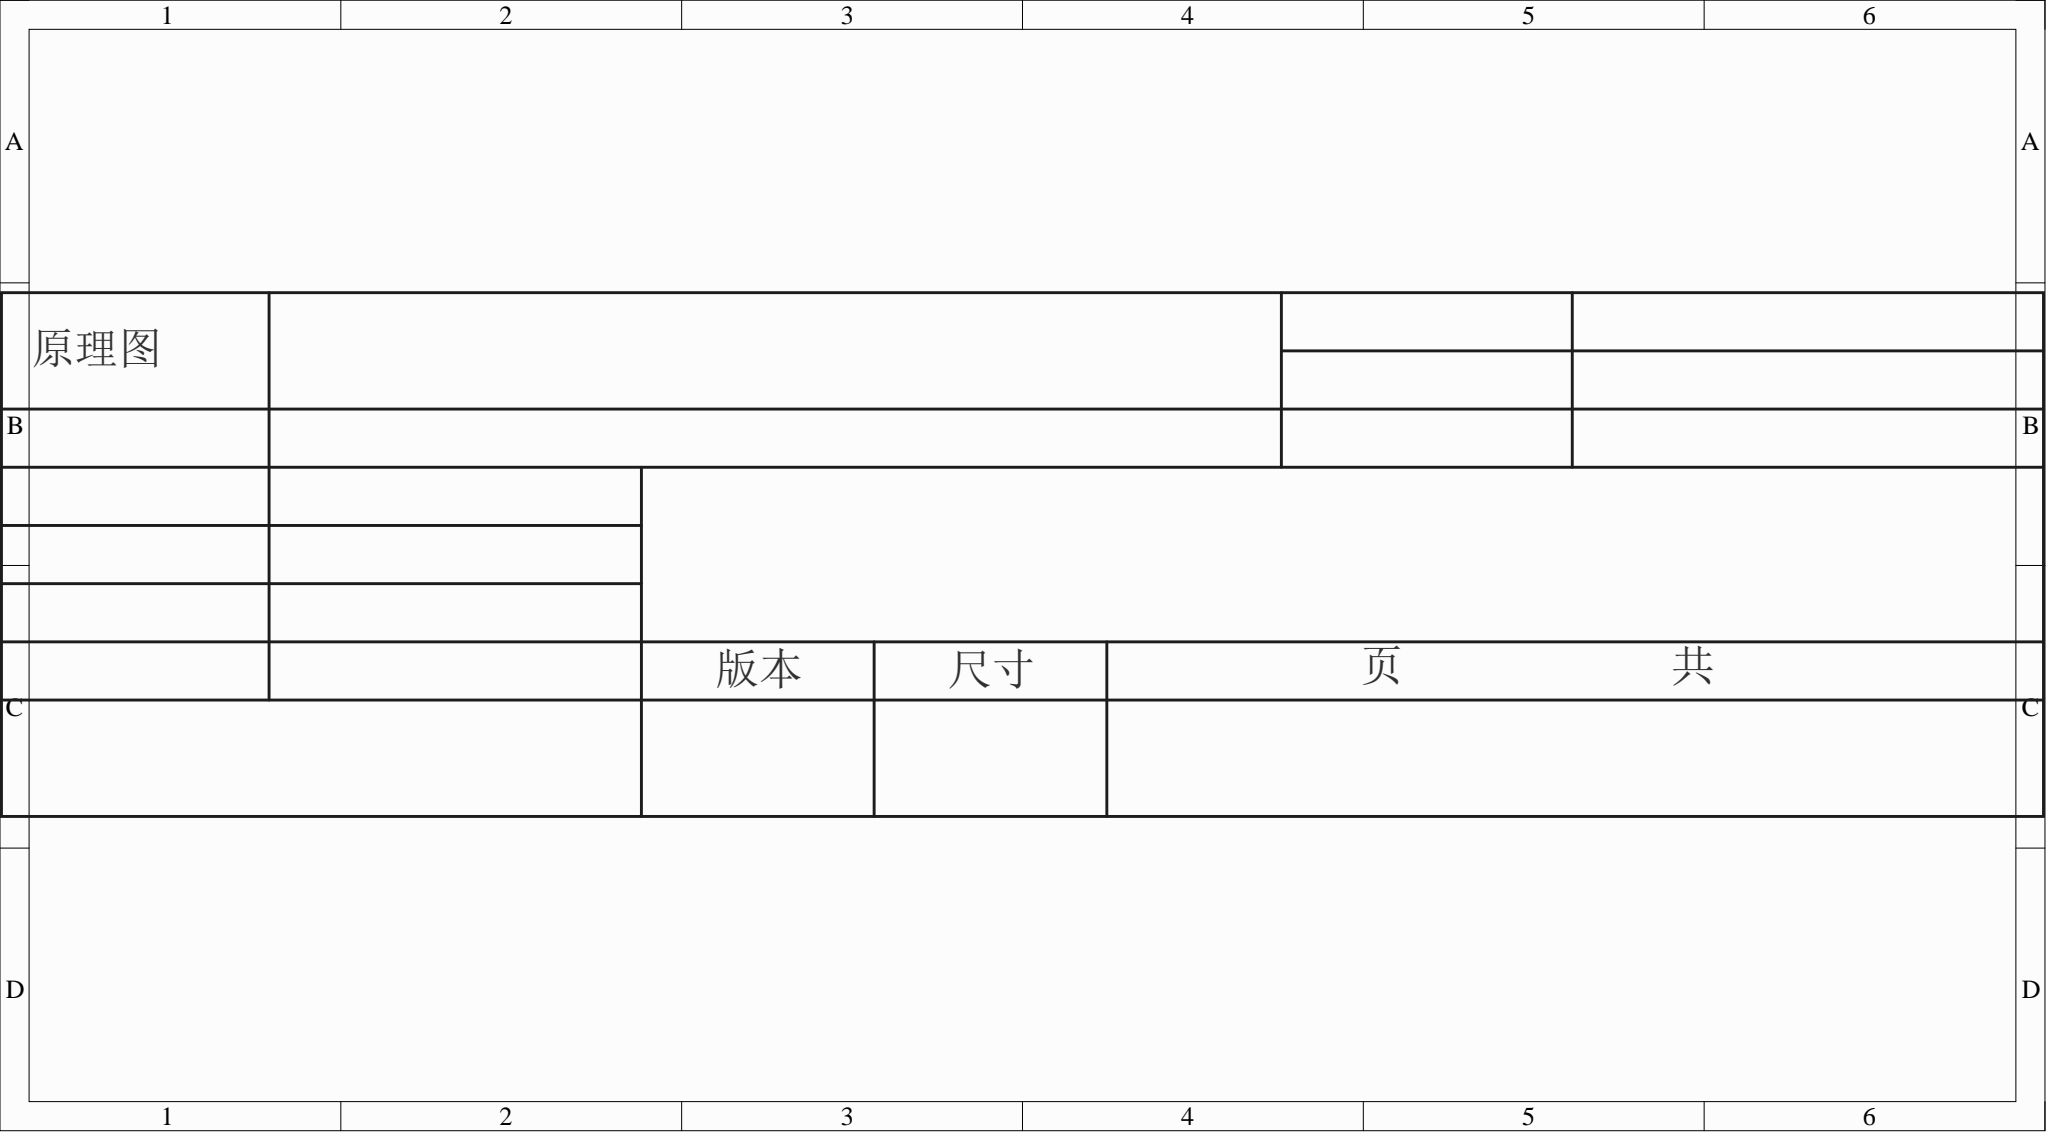Circuit board | Altium Designer | 22 parts | 41 nets
Bill of materials:
Comment,Description,Designator,Footprint,LibRef,Quantity
"1uF","","C1","C0805","CAP_0805","1"
"10nF","","C2","C0805","CAP_0805","1"
"","","H1","HDR-TH_2P-P2.54-V-M-1","HDR-M_2.54_1x2P","1"
"","","H8, H9, H10, H11, H12, H13","HDR-TH_6P-P2.54-V-M-1","HDR-M_2.54_1x6P","6"
"轻触按键3*4*H","","J8","SW-SMD_L4.0-W2.9-LS5.0","轻触按键3*4*H","1"
"10k","","R1","R0603","Res_0603","1"
"2.2k","","R2","R0603","Res_0603","1"
"开关","","SW1","SW-TH_SS-12D01-GX","开关","1"
"NE555PE4","单精度计时器 8-PDIP 0 to 70","U8","PDIP-8_L9.6-W6.4-P2.54-LS7.9-BL-1","NE555PE4","1"
"74LS160D","工作电压:2V~6V;元件数:1;触发沿:上升沿;计数速率:24MHz;","U68, U69, U77, U78, U81, U82","PDIP-16_L19.3-W6.4-P2.54-LS7.94-BL","SN74LS192N(LX)","6"
"SN74LS08DR(LX)","逻辑类型:与门;通道数:4;电源电压:2V~6V;静态电流(最大值):2uA;最大传播延迟:15ns@6V;","U85","SOIC-14_L8.7-W3.9-P1.27-LS6.0-BL","SN74LS08DR(LX)","1"
"SN74LS00N(LX)","逻辑类型:与非门;通道数:4;电源电压:2V~6V;静态电流(最大值):2uA;最大传播延迟:7ns@6V;","U86","PDIP-14_L19.3-W6.4-P2.54-LS7.9-BL","SN74LS00N(LX)","1"
Netlist (Protel format):
[
C1
C0805
1uF



]
[
C2
C0805
10nF



]
[
H1
HDR-TH_2P-P2.54-V-M-1




]
[
H8
HDR-TH_6P-P2.54-V-M-1




]
[
H9
HDR-TH_6P-P2.54-V-M-1




]
[
H10
HDR-TH_6P-P2.54-V-M-1




]
[
H11
HDR-TH_6P-P2.54-V-M-1




]
[
H12
HDR-TH_6P-P2.54-V-M-1




]
[
H13
HDR-TH_6P-P2.54-V-M-1




]
[
J8
SW-SMD_L4.0-W2.9-LS5.0
轻触按键3*4*H



]
[
R1
R0603
10k



]
[
R2
R0603
2.2k



]
[
SW1
SW-TH_SS-12D01-GX
开关



]
[
U8
PDIP-8_L9.6-W6.4-P2.54-LS7.9-BL-1
NE555PE4



]
[
U68
PDIP-16_L19.3-W6.4-P2.54-LS7.94-BL
74LS160D



]
[
U69
PDIP-16_L19.3-W6.4-P2.54-LS7.94-BL
74LS160D



]
[
U77
PDIP-16_L19.3-W6.4-P2.54-LS7.94-BL
74LS160D



]
[
U78
PDIP-16_L19.3-W6.4-P2.54-LS7.94-BL
74LS160D



]
[
U81
PDIP-16_L19.3-W6.4-P2.54-LS7.94-BL
74LS160D



]
[
U82
PDIP-16_L19.3-W6.4-P2.54-LS7.94-BL
74LS160D



]
[
U85
SOIC-14_L8.7-W3.9-P1.27-LS6.0-BL
SN74LS08DR(LX)



]
[
U86
PDIP-14_L19.3-W6.4-P2.54-LS7.9-BL
SN74LS00N(LX)



]
(
VCC
H1-1
H8-5
H9-5
H10-5
H11-5
H12-5
H13-5
R1-2
SW1-1
U8-4
U8-8
U68-7
U68-9
U68-10
U68-16
U69-7
U69-9
U69-10
U69-16
U77-7
U77-9
U77-10
U77-16
U78-7
U78-9
U78-10
U78-16
U81-7
U81-9
U81-10
U81-16
U82-7
U82-9
U82-10
U82-16
U85-14
U86-14
)
(
NetU85_10
U85-10
U86-8
)
(
NetU85_2
U85-2
U86-6
)
(
NetU81_2
U81-2
U82-15
)
(
NetU81_1
U81-1
U85-3
)
(
NetU77_15
U77-15
U82-2
)
(
NetU77_2
U77-2
U78-15
)
(
NetU77_1
U77-1
U82-1
U85-8
)
(
NetU68_15
U68-15
U78-2
)
(
NetU68_2
U68-2
U69-15
)
(
NetSW1_2
SW1-2
U68-1
U69-2
U78-1
U85-1
U85-9
)
(
NetR1_1
R1-1
R2-2
U8-7
)
(
NetJ8_2
J8-2
U69-1
)
(
NetJ8_1
J8-1
U8-3
)
(
NetH13_4
H13-4
U69-11
)
(
NetH13_3
H13-3
U69-12
)
(
NetH13_2
H13-2
U69-13
)
(
NetH13_1
H13-1
U69-14
)
(
NetH12_4
H12-4
U68-11
)
(
NetH12_3
H12-3
U68-12
)
(
NetH12_2
H12-2
U68-13
)
(
NetH12_1
H12-1
U68-14
)
(
NetH11_4
H11-4
U78-11
)
(
NetH11_3
H11-3
U78-12
)
(
NetH11_2
H11-2
U78-13
)
(
NetH11_1
H11-1
U78-14
)
(
NetH10_4
H10-4
U77-11
)
(
NetH10_3
H10-3
U77-12
U86-9
)
(
NetH10_2
H10-2
U77-13
U86-10
)
(
NetH10_1
H10-1
U77-14
)
(
NetH9_4
H9-4
U82-11
)
(
NetH9_3
H9-3
U82-12
)
(
NetH9_2
H9-2
U82-13
)
(
NetH9_1
H9-1
U82-14
)
(
NetH8_4
H8-4
U81-11
)
(
NetH8_3
H8-3
U81-12
U86-5
)
(
NetH8_2
H8-2
U81-13
U86-4
)
(
NetH8_1
H8-1
U81-14
)
(
NetC2_2
C2-2
U8-5
)
(
NetC1_2
C1-2
R2-1
U8-2
U8-6
)
(
GND
C1-1
C2-1
H1-2
H8-6
H9-6
H10-6
H11-6
H12-6
H13-6
SW1-3
U8-1
U68-3
U68-4
U68-5
U68-6
U68-8
U69-3
U69-4
U69-5
U69-6
U69-8
U77-3
U77-4
U77-5
U77-6
U77-8
U78-3
U78-4
U78-5
U78-6
U78-8
U81-3
U81-4
U81-5
U81-6
U81-8
U82-3
U82-4
U82-5
U82-6
U82-8
U85-7
U86-7
)